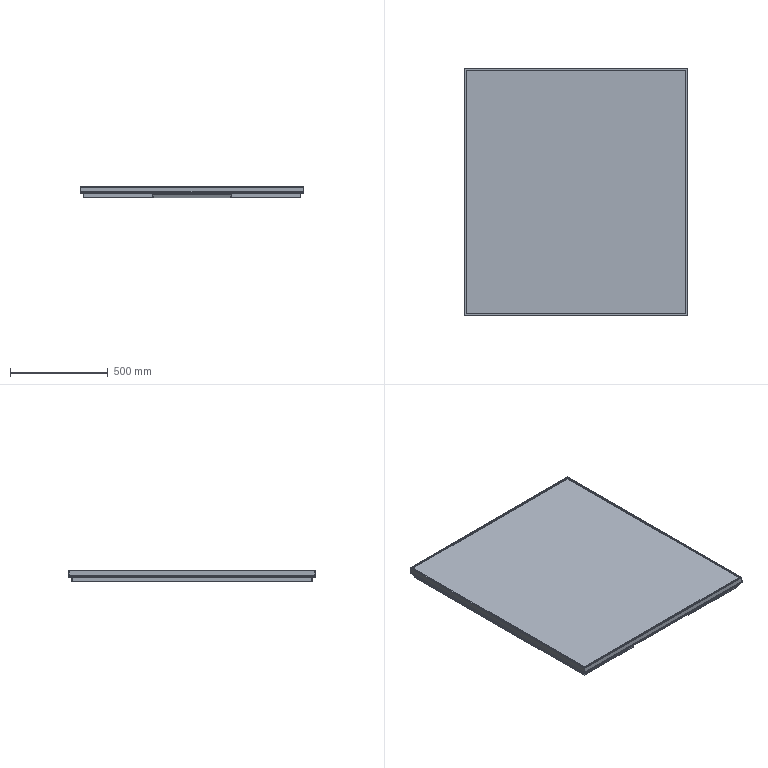Part | SolidWorks | 7 solids | 264 faces | box 1140 x 1260 x 60.087 mm | volume 6458843 mm3 | plane 176 | cylinder 76 | spline 12 | commonest cylinder face diameters 7 x30 11 x16 0.4 x9 2.4 x9 2 x6 1 x4